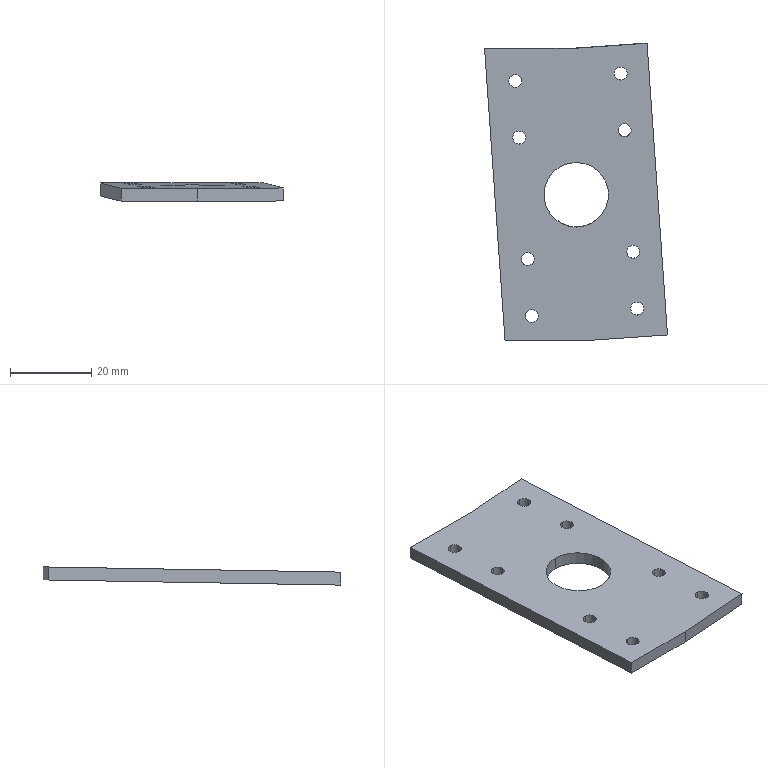Part | SolidWorks | features BaseBody 1 | 1 solid | 26 faces | box 45.033 x 73.349 x 4.479 mm | volume 8385 mm3 | cylinder 18 | plane 8 | commonest cylinder face diameters 3.2 x16 15.9 x2
STEP:
#1=CARTESIAN_POINT('',(17.015,-2.731,-4.048));
#2=VERTEX_POINT('',#1);
#3=CARTESIAN_POINT('',(17.015,0.4687,-3.992));
#4=VERTEX_POINT('',#3);
#5=CARTESIAN_POINT('',(17.015,-1.131,-4.02));
#6=DIRECTION('',(0.,0.01745,-0.9998));
#7=DIRECTION('',(0.,-0.9998,-0.01745));
#8=AXIS2_PLACEMENT_3D('',#5,#6,#7);
#9=CIRCLE('',#8,1.6);
#10=EDGE_CURVE('',#2,#4,#9,.T.);
#11=ORIENTED_EDGE('',*,*,#10,.T.);
#12=CARTESIAN_POINT('',(17.015,0.4129,-0.7929));
#13=VERTEX_POINT('',#12);
#14=CARTESIAN_POINT('',(17.015,0.4687,-3.992));
#15=DIRECTION('',(0.,-0.01745,0.9998));
#16=VECTOR('',#15,1000.);
#17=LINE('',#14,#16);
#18=EDGE_CURVE('',#4,#13,#17,.T.);
#19=ORIENTED_EDGE('',*,*,#18,.T.);
#20=CARTESIAN_POINT('',(17.015,-2.787,-0.8488));
#21=VERTEX_POINT('',#20);
#22=CARTESIAN_POINT('',(17.015,-1.187,-0.8208));
#23=DIRECTION('',(0.,-0.01745,0.9998));
#24=DIRECTION('',(0.,-0.9998,-0.01745));
#25=AXIS2_PLACEMENT_3D('',#22,#23,#24);
#26=CIRCLE('',#25,1.6);
#27=EDGE_CURVE('',#13,#21,#26,.T.);
#28=ORIENTED_EDGE('',*,*,#27,.T.);
#29=CARTESIAN_POINT('',(17.015,-2.731,-4.048));
#30=DIRECTION('',(0.,-0.01745,0.9998));
#31=VECTOR('',#30,1000.);
#32=LINE('',#29,#31);
#33=EDGE_CURVE('',#2,#21,#32,.T.);
#34=ORIENTED_EDGE('',*,*,#33,.F.);
#35=EDGE_LOOP('',(#11,#19,#28,#34));
#36=FACE_OUTER_BOUND('',#35,.T.);
#37=CARTESIAN_POINT('',(17.015,-1.131,-4.02));
#38=DIRECTION('',(0.,-0.01745,0.9998));
#39=DIRECTION('',(0.,-0.9998,-0.01745));
#40=AXIS2_PLACEMENT_3D('',#37,#38,#39);
#41=CYLINDRICAL_SURFACE('',#40,1.6);
#42=ADVANCED_FACE('',(#36),#41,.F.);
#43=CARTESIAN_POINT('',(-7.944,-15.31,-4.268));
#44=VERTEX_POINT('',#43);
#45=CARTESIAN_POINT('',(-7.944,-18.51,-4.324));
#46=VERTEX_POINT('',#45);
#47=CARTESIAN_POINT('',(-7.944,-16.91,-4.296));
#48=DIRECTION('',(0.,-0.01745,0.9998));
#49=DIRECTION('',(0.,-0.9998,-0.01745));
#50=AXIS2_PLACEMENT_3D('',#47,#48,#49);
#51=CIRCLE('',#50,1.6);
#52=EDGE_CURVE('',#44,#46,#51,.T.);
#53=ORIENTED_EDGE('',*,*,#52,.F.);
#54=CARTESIAN_POINT('',(-7.944,-15.366,-1.068));
#55=VERTEX_POINT('',#54);
#56=CARTESIAN_POINT('',(-7.944,-15.31,-4.268));
#57=DIRECTION('',(0.,-0.01745,0.9998));
#58=VECTOR('',#57,1000.);
#59=LINE('',#56,#58);
#60=EDGE_CURVE('',#44,#55,#59,.T.);
#61=ORIENTED_EDGE('',*,*,#60,.T.);
#62=CARTESIAN_POINT('',(-7.944,-18.565,-1.124));
#63=VERTEX_POINT('',#62);
#64=CARTESIAN_POINT('',(-7.944,-16.966,-1.096));
#65=DIRECTION('',(0.,-0.01745,0.9998));
#66=DIRECTION('',(0.,-0.9998,-0.01745));
#67=AXIS2_PLACEMENT_3D('',#64,#65,#66);
#68=CIRCLE('',#67,1.6);
#69=EDGE_CURVE('',#55,#63,#68,.T.);
#70=ORIENTED_EDGE('',*,*,#69,.T.);
#71=CARTESIAN_POINT('',(-7.944,-18.51,-4.324));
#72=DIRECTION('',(0.,-0.01745,0.9998));
#73=VECTOR('',#72,1000.);
#74=LINE('',#71,#73);
#75=EDGE_CURVE('',#46,#63,#74,.T.);
#76=ORIENTED_EDGE('',*,*,#75,.F.);
#77=EDGE_LOOP('',(#53,#61,#70,#76));
#78=FACE_OUTER_BOUND('',#77,.T.);
#79=CARTESIAN_POINT('',(-7.944,-16.91,-4.296));
#80=DIRECTION('',(0.,-0.01745,0.9998));
#81=DIRECTION('',(0.,-0.9998,-0.01745));
#82=AXIS2_PLACEMENT_3D('',#79,#80,#81);
#83=CYLINDRICAL_SURFACE('',#82,1.6);
#84=ADVANCED_FACE('',(#78),#83,.F.);
#85=CARTESIAN_POINT('',(3.,20.869,-3.636));
#86=VERTEX_POINT('',#85);
#87=CARTESIAN_POINT('',(3.,4.971,-3.914));
#88=VERTEX_POINT('',#87);
#89=CARTESIAN_POINT('',(3.,12.92,-3.775));
#90=DIRECTION('',(0.,-0.01745,0.9998));
#91=DIRECTION('',(0.,-0.9998,-0.01745));
#92=AXIS2_PLACEMENT_3D('',#89,#90,#91);
#93=CIRCLE('',#92,7.95);
#94=EDGE_CURVE('',#86,#88,#93,.T.);
#95=ORIENTED_EDGE('',*,*,#94,.F.);
#96=CARTESIAN_POINT('',(3.,20.813,-0.4368));
#97=VERTEX_POINT('',#96);
#98=CARTESIAN_POINT('',(3.,20.869,-3.636));
#99=DIRECTION('',(0.,-0.01745,0.9998));
#100=VECTOR('',#99,1000.);
#101=LINE('',#98,#100);
#102=EDGE_CURVE('',#86,#97,#101,.T.);
#103=ORIENTED_EDGE('',*,*,#102,.T.);
#104=CARTESIAN_POINT('',(3.,4.916,-0.7143));
#105=VERTEX_POINT('',#104);
#106=CARTESIAN_POINT('',(3.,12.864,-0.5756));
#107=DIRECTION('',(0.,-0.01745,0.9998));
#108=DIRECTION('',(0.,-0.9998,-0.01745));
#109=AXIS2_PLACEMENT_3D('',#106,#107,#108);
#110=CIRCLE('',#109,7.95);
#111=EDGE_CURVE('',#97,#105,#110,.T.);
#112=ORIENTED_EDGE('',*,*,#111,.T.);
#113=CARTESIAN_POINT('',(3.,4.971,-3.914));
#114=DIRECTION('',(0.,-0.01745,0.9998));
#115=VECTOR('',#114,1000.);
#116=LINE('',#113,#115);
#117=EDGE_CURVE('',#88,#105,#116,.T.);
#118=ORIENTED_EDGE('',*,*,#117,.F.);
#119=EDGE_LOOP('',(#95,#103,#112,#118));
#120=FACE_OUTER_BOUND('',#119,.T.);
#121=CARTESIAN_POINT('',(3.,12.92,-3.775));
#122=DIRECTION('',(0.,-0.01745,0.9998));
#123=DIRECTION('',(0.,-0.9998,-0.01745));
#124=AXIS2_PLACEMENT_3D('',#121,#122,#123);
#125=CYLINDRICAL_SURFACE('',#124,7.95);
#126=ADVANCED_FACE('',(#120),#125,.F.);
#127=CARTESIAN_POINT('',(-11.015,28.571,-3.502));
#128=VERTEX_POINT('',#127);
#129=CARTESIAN_POINT('',(-11.015,25.372,-3.558));
#130=VERTEX_POINT('',#129);
#131=CARTESIAN_POINT('',(-11.015,26.972,-3.53));
#132=DIRECTION('',(0.,-0.01745,0.9998));
#133=DIRECTION('',(0.,-0.9998,-0.01745));
#134=AXIS2_PLACEMENT_3D('',#131,#132,#133);
#135=CIRCLE('',#134,1.6);
#136=EDGE_CURVE('',#128,#130,#135,.T.);
#137=ORIENTED_EDGE('',*,*,#136,.F.);
#138=CARTESIAN_POINT('',(-11.015,28.515,-0.3024));
#139=VERTEX_POINT('',#138);
#140=CARTESIAN_POINT('',(-11.015,28.571,-3.502));
#141=DIRECTION('',(0.,-0.01745,0.9998));
#142=VECTOR('',#141,1000.);
#143=LINE('',#140,#142);
#144=EDGE_CURVE('',#128,#139,#143,.T.);
#145=ORIENTED_EDGE('',*,*,#144,.T.);
#146=CARTESIAN_POINT('',(-11.015,25.316,-0.3582));
#147=VERTEX_POINT('',#146);
#148=CARTESIAN_POINT('',(-11.015,26.916,-0.3303));
#149=DIRECTION('',(0.,-0.01745,0.9998));
#150=DIRECTION('',(0.,-0.9998,-0.01745));
#151=AXIS2_PLACEMENT_3D('',#148,#149,#150);
#152=CIRCLE('',#151,1.6);
#153=EDGE_CURVE('',#139,#147,#152,.T.);
#154=ORIENTED_EDGE('',*,*,#153,.T.);
#155=CARTESIAN_POINT('',(-11.015,25.372,-3.558));
#156=DIRECTION('',(0.,-0.01745,0.9998));
#157=VECTOR('',#156,1000.);
#158=LINE('',#155,#157);
#159=EDGE_CURVE('',#130,#147,#158,.T.);
#160=ORIENTED_EDGE('',*,*,#159,.F.);
#161=EDGE_LOOP('',(#137,#145,#154,#160));
#162=FACE_OUTER_BOUND('',#161,.T.);
#163=CARTESIAN_POINT('',(-11.015,26.972,-3.53));
#164=DIRECTION('',(0.,-0.01745,0.9998));
#165=DIRECTION('',(0.,-0.9998,-0.01745));
#166=AXIS2_PLACEMENT_3D('',#163,#164,#165);
#167=CYLINDRICAL_SURFACE('',#166,1.6);
#168=ADVANCED_FACE('',(#162),#167,.F.);
#169=CARTESIAN_POINT('',(13.944,44.35,-3.226));
#170=VERTEX_POINT('',#169);
#171=CARTESIAN_POINT('',(13.944,41.151,-3.282));
#172=VERTEX_POINT('',#171);
#173=CARTESIAN_POINT('',(13.944,42.75,-3.254));
#174=DIRECTION('',(0.,-0.01745,0.9998));
#175=DIRECTION('',(0.,-0.9998,-0.01745));
#176=AXIS2_PLACEMENT_3D('',#173,#174,#175);
#177=CIRCLE('',#176,1.6);
#178=EDGE_CURVE('',#170,#172,#177,.T.);
#179=ORIENTED_EDGE('',*,*,#178,.F.);
#180=CARTESIAN_POINT('',(13.944,44.294,-0.02696));
#181=VERTEX_POINT('',#180);
#182=CARTESIAN_POINT('',(13.944,44.35,-3.226));
#183=DIRECTION('',(0.,-0.01745,0.9998));
#184=VECTOR('',#183,1000.);
#185=LINE('',#182,#184);
#186=EDGE_CURVE('',#170,#181,#185,.T.);
#187=ORIENTED_EDGE('',*,*,#186,.T.);
#188=CARTESIAN_POINT('',(13.944,41.095,-0.08281));
#189=VERTEX_POINT('',#188);
#190=CARTESIAN_POINT('',(13.944,42.695,-0.05489));
#191=DIRECTION('',(0.,-0.01745,0.9998));
#192=DIRECTION('',(0.,-0.9998,-0.01745));
#193=AXIS2_PLACEMENT_3D('',#190,#191,#192);
#194=CIRCLE('',#193,1.6);
#195=EDGE_CURVE('',#181,#189,#194,.T.);
#196=ORIENTED_EDGE('',*,*,#195,.T.);
#197=CARTESIAN_POINT('',(13.944,41.151,-3.282));
#198=DIRECTION('',(0.,-0.01745,0.9998));
#199=VECTOR('',#198,1000.);
#200=LINE('',#197,#199);
#201=EDGE_CURVE('',#172,#189,#200,.T.);
#202=ORIENTED_EDGE('',*,*,#201,.F.);
#203=EDGE_LOOP('',(#179,#187,#196,#202));
#204=FACE_OUTER_BOUND('',#203,.T.);
#205=CARTESIAN_POINT('',(13.944,42.75,-3.254));
#206=DIRECTION('',(0.,-0.01745,0.9998));
#207=DIRECTION('',(0.,-0.9998,-0.01745));
#208=AXIS2_PLACEMENT_3D('',#205,#206,#207);
#209=CYLINDRICAL_SURFACE('',#208,1.6);
#210=ADVANCED_FACE('',(#204),#209,.F.);
#211=CARTESIAN_POINT('',(-11.993,42.535,-3.258));
#212=VERTEX_POINT('',#211);
#213=CARTESIAN_POINT('',(-11.993,39.336,-3.314));
#214=VERTEX_POINT('',#213);
#215=CARTESIAN_POINT('',(-11.993,40.935,-3.286));
#216=DIRECTION('',(0.,-0.01745,0.9998));
#217=DIRECTION('',(0.,-0.9998,-0.01745));
#218=AXIS2_PLACEMENT_3D('',#215,#216,#217);
#219=CIRCLE('',#218,1.6);
#220=EDGE_CURVE('',#212,#214,#219,.T.);
#221=ORIENTED_EDGE('',*,*,#220,.F.);
#222=CARTESIAN_POINT('',(-11.993,42.479,-0.05864));
#223=VERTEX_POINT('',#222);
#224=CARTESIAN_POINT('',(-11.993,42.535,-3.258));
#225=DIRECTION('',(0.,-0.01745,0.9998));
#226=VECTOR('',#225,1000.);
#227=LINE('',#224,#226);
#228=EDGE_CURVE('',#212,#223,#227,.T.);
#229=ORIENTED_EDGE('',*,*,#228,.T.);
#230=CARTESIAN_POINT('',(-11.993,39.28,-0.1145));
#231=VERTEX_POINT('',#230);
#232=CARTESIAN_POINT('',(-11.993,40.879,-0.08657));
#233=DIRECTION('',(0.,-0.01745,0.9998));
#234=DIRECTION('',(0.,-0.9998,-0.01745));
#235=AXIS2_PLACEMENT_3D('',#232,#233,#234);
#236=CIRCLE('',#235,1.6);
#237=EDGE_CURVE('',#223,#231,#236,.T.);
#238=ORIENTED_EDGE('',*,*,#237,.T.);
#239=CARTESIAN_POINT('',(-11.993,39.336,-3.314));
#240=DIRECTION('',(0.,-0.01745,0.9998));
#241=VECTOR('',#240,1000.);
#242=LINE('',#239,#241);
#243=EDGE_CURVE('',#214,#231,#242,.T.);
#244=ORIENTED_EDGE('',*,*,#243,.F.);
#245=EDGE_LOOP('',(#221,#229,#238,#244));
#246=FACE_OUTER_BOUND('',#245,.T.);
#247=CARTESIAN_POINT('',(-11.993,40.935,-3.286));
#248=DIRECTION('',(0.,-0.01745,0.9998));
#249=DIRECTION('',(0.,-0.9998,-0.01745));
#250=AXIS2_PLACEMENT_3D('',#247,#248,#249);
#251=CYLINDRICAL_SURFACE('',#250,1.6);
#252=ADVANCED_FACE('',(#246),#251,.F.);
#253=CARTESIAN_POINT('',(14.921,30.386,-3.47));
#254=VERTEX_POINT('',#253);
#255=CARTESIAN_POINT('',(14.921,27.187,-3.526));
#256=VERTEX_POINT('',#255);
#257=CARTESIAN_POINT('',(14.921,28.787,-3.498));
#258=DIRECTION('',(0.,-0.01745,0.9998));
#259=DIRECTION('',(0.,-0.9998,-0.01745));
#260=AXIS2_PLACEMENT_3D('',#257,#258,#259);
#261=CIRCLE('',#260,1.6);
#262=EDGE_CURVE('',#254,#256,#261,.T.);
#263=ORIENTED_EDGE('',*,*,#262,.F.);
#264=CARTESIAN_POINT('',(14.921,30.331,-0.2707));
#265=VERTEX_POINT('',#264);
#266=CARTESIAN_POINT('',(14.921,30.386,-3.47));
#267=DIRECTION('',(0.,-0.01745,0.9998));
#268=VECTOR('',#267,1000.);
#269=LINE('',#266,#268);
#270=EDGE_CURVE('',#254,#265,#269,.T.);
#271=ORIENTED_EDGE('',*,*,#270,.T.);
#272=CARTESIAN_POINT('',(14.921,27.131,-0.3265));
#273=VERTEX_POINT('',#272);
#274=CARTESIAN_POINT('',(14.921,28.731,-0.2986));
#275=DIRECTION('',(0.,-0.01745,0.9998));
#276=DIRECTION('',(0.,-0.9998,-0.01745));
#277=AXIS2_PLACEMENT_3D('',#274,#275,#276);
#278=CIRCLE('',#277,1.6);
#279=EDGE_CURVE('',#265,#273,#278,.T.);
#280=ORIENTED_EDGE('',*,*,#279,.T.);
#281=CARTESIAN_POINT('',(14.921,27.187,-3.526));
#282=DIRECTION('',(0.,-0.01745,0.9998));
#283=VECTOR('',#282,1000.);
#284=LINE('',#281,#283);
#285=EDGE_CURVE('',#256,#273,#284,.T.);
#286=ORIENTED_EDGE('',*,*,#285,.F.);
#287=EDGE_LOOP('',(#263,#271,#280,#286));
#288=FACE_OUTER_BOUND('',#287,.T.);
#289=CARTESIAN_POINT('',(14.921,28.787,-3.498));
#290=DIRECTION('',(0.,-0.01745,0.9998));
#291=DIRECTION('',(0.,-0.9998,-0.01745));
#292=AXIS2_PLACEMENT_3D('',#289,#290,#291);
#293=CYLINDRICAL_SURFACE('',#292,1.6);
#294=ADVANCED_FACE('',(#288),#293,.F.);
#295=CARTESIAN_POINT('',(-8.921,-1.346,-4.024));
#296=VERTEX_POINT('',#295);
#297=CARTESIAN_POINT('',(-8.921,-4.546,-4.08));
#298=VERTEX_POINT('',#297);
#299=CARTESIAN_POINT('',(-8.921,-2.946,-4.052));
#300=DIRECTION('',(0.,-0.01745,0.9998));
#301=DIRECTION('',(0.,-0.9998,-0.01745));
#302=AXIS2_PLACEMENT_3D('',#299,#300,#301);
#303=CIRCLE('',#302,1.6);
#304=EDGE_CURVE('',#296,#298,#303,.T.);
#305=ORIENTED_EDGE('',*,*,#304,.F.);
#306=CARTESIAN_POINT('',(-8.921,-1.402,-0.8246));
#307=VERTEX_POINT('',#306);
#308=CARTESIAN_POINT('',(-8.921,-1.346,-4.024));
#309=DIRECTION('',(0.,-0.01745,0.9998));
#310=VECTOR('',#309,1000.);
#311=LINE('',#308,#310);
#312=EDGE_CURVE('',#296,#307,#311,.T.);
#313=ORIENTED_EDGE('',*,*,#312,.T.);
#314=CARTESIAN_POINT('',(-8.921,-4.602,-0.8804));
#315=VERTEX_POINT('',#314);
#316=CARTESIAN_POINT('',(-8.921,-3.002,-0.8525));
#317=DIRECTION('',(0.,-0.01745,0.9998));
#318=DIRECTION('',(0.,-0.9998,-0.01745));
#319=AXIS2_PLACEMENT_3D('',#316,#317,#318);
#320=CIRCLE('',#319,1.6);
#321=EDGE_CURVE('',#307,#315,#320,.T.);
#322=ORIENTED_EDGE('',*,*,#321,.T.);
#323=CARTESIAN_POINT('',(-8.921,-4.546,-4.08));
#324=DIRECTION('',(0.,-0.01745,0.9998));
#325=VECTOR('',#324,1000.);
#326=LINE('',#323,#325);
#327=EDGE_CURVE('',#298,#315,#326,.T.);
#328=ORIENTED_EDGE('',*,*,#327,.F.);
#329=EDGE_LOOP('',(#305,#313,#322,#328));
#330=FACE_OUTER_BOUND('',#329,.T.);
#331=CARTESIAN_POINT('',(-8.921,-2.946,-4.052));
#332=DIRECTION('',(0.,-0.01745,0.9998));
#333=DIRECTION('',(0.,-0.9998,-0.01745));
#334=AXIS2_PLACEMENT_3D('',#331,#332,#333);
#335=CYLINDRICAL_SURFACE('',#334,1.6);
#336=ADVANCED_FACE('',(#330),#335,.F.);
#337=CARTESIAN_POINT('',(17.993,-13.495,-4.236));
#338=VERTEX_POINT('',#337);
#339=CARTESIAN_POINT('',(17.993,-16.694,-4.292));
#340=VERTEX_POINT('',#339);
#341=CARTESIAN_POINT('',(17.993,-15.095,-4.264));
#342=DIRECTION('',(0.,-0.01745,0.9998));
#343=DIRECTION('',(0.,-0.9998,-0.01745));
#344=AXIS2_PLACEMENT_3D('',#341,#342,#343);
#345=CIRCLE('',#344,1.6);
#346=EDGE_CURVE('',#338,#340,#345,.T.);
#347=ORIENTED_EDGE('',*,*,#346,.F.);
#348=CARTESIAN_POINT('',(17.993,-13.551,-1.037));
#349=VERTEX_POINT('',#348);
#350=CARTESIAN_POINT('',(17.993,-13.495,-4.236));
#351=DIRECTION('',(0.,-0.01745,0.9998));
#352=VECTOR('',#351,1000.);
#353=LINE('',#350,#352);
#354=EDGE_CURVE('',#338,#349,#353,.T.);
#355=ORIENTED_EDGE('',*,*,#354,.T.);
#356=CARTESIAN_POINT('',(17.993,-16.75,-1.093));
#357=VERTEX_POINT('',#356);
#358=CARTESIAN_POINT('',(17.993,-15.151,-1.065));
#359=DIRECTION('',(0.,-0.01745,0.9998));
#360=DIRECTION('',(0.,-0.9998,-0.01745));
#361=AXIS2_PLACEMENT_3D('',#358,#359,#360);
#362=CIRCLE('',#361,1.6);
#363=EDGE_CURVE('',#349,#357,#362,.T.);
#364=ORIENTED_EDGE('',*,*,#363,.T.);
#365=CARTESIAN_POINT('',(17.993,-16.694,-4.292));
#366=DIRECTION('',(0.,-0.01745,0.9998));
#367=VECTOR('',#366,1000.);
#368=LINE('',#365,#367);
#369=EDGE_CURVE('',#340,#357,#368,.T.);
#370=ORIENTED_EDGE('',*,*,#369,.F.);
#371=EDGE_LOOP('',(#347,#355,#364,#370));
#372=FACE_OUTER_BOUND('',#371,.T.);
#373=CARTESIAN_POINT('',(17.993,-15.095,-4.264));
#374=DIRECTION('',(0.,-0.01745,0.9998));
#375=DIRECTION('',(0.,-0.9998,-0.01745));
#376=AXIS2_PLACEMENT_3D('',#373,#374,#375);
#377=CYLINDRICAL_SURFACE('',#376,1.6);
#378=ADVANCED_FACE('',(#372),#377,.F.);
#379=ORIENTED_EDGE('',*,*,#18,.F.);
#380=CARTESIAN_POINT('',(17.015,-1.131,-4.02));
#381=DIRECTION('',(0.,0.01745,-0.9998));
#382=DIRECTION('',(0.,-0.9998,-0.01745));
#383=AXIS2_PLACEMENT_3D('',#380,#381,#382);
#384=CIRCLE('',#383,1.6);
#385=EDGE_CURVE('',#4,#2,#384,.T.);
#386=ORIENTED_EDGE('',*,*,#385,.T.);
#387=ORIENTED_EDGE('',*,*,#33,.T.);
#388=CARTESIAN_POINT('',(17.015,-1.187,-0.8208));
#389=DIRECTION('',(0.,-0.01745,0.9998));
#390=DIRECTION('',(0.,-0.9998,-0.01745));
#391=AXIS2_PLACEMENT_3D('',#388,#389,#390);
#392=CIRCLE('',#391,1.6);
#393=EDGE_CURVE('',#21,#13,#392,.T.);
#394=ORIENTED_EDGE('',*,*,#393,.T.);
#395=EDGE_LOOP('',(#379,#386,#387,#394));
#396=FACE_OUTER_BOUND('',#395,.T.);
#397=CARTESIAN_POINT('',(17.015,-1.131,-4.02));
#398=DIRECTION('',(0.,-0.01745,0.9998));
#399=DIRECTION('',(0.,-0.9998,-0.01745));
#400=AXIS2_PLACEMENT_3D('',#397,#398,#399);
#401=CYLINDRICAL_SURFACE('',#400,1.6);
#402=ADVANCED_FACE('',(#396),#401,.F.);
#403=ORIENTED_EDGE('',*,*,#393,.F.);
#404=ORIENTED_EDGE('',*,*,#27,.F.);
#405=EDGE_LOOP('',(#403,#404));
#406=FACE_BOUND('',#405,.T.);
#407=CARTESIAN_POINT('',(-7.944,-16.966,-1.096));
#408=DIRECTION('',(0.,-0.01745,0.9998));
#409=DIRECTION('',(0.,-0.9998,-0.01745));
#410=AXIS2_PLACEMENT_3D('',#407,#408,#409);
#411=CIRCLE('',#410,1.6);
#412=EDGE_CURVE('',#63,#55,#411,.T.);
#413=ORIENTED_EDGE('',*,*,#412,.F.);
#414=ORIENTED_EDGE('',*,*,#69,.F.);
#415=EDGE_LOOP('',(#413,#414));
#416=FACE_BOUND('',#415,.T.);
#417=CARTESIAN_POINT('',(3.,12.864,-0.5756));
#418=DIRECTION('',(0.,-0.01745,0.9998));
#419=DIRECTION('',(0.,-0.9998,-0.01745));
#420=AXIS2_PLACEMENT_3D('',#417,#418,#419);
#421=CIRCLE('',#420,7.95);
#422=EDGE_CURVE('',#105,#97,#421,.T.);
#423=ORIENTED_EDGE('',*,*,#422,.F.);
#424=ORIENTED_EDGE('',*,*,#111,.F.);
#425=EDGE_LOOP('',(#423,#424));
#426=FACE_BOUND('',#425,.T.);
#427=CARTESIAN_POINT('',(-11.015,26.916,-0.3303));
#428=DIRECTION('',(0.,-0.01745,0.9998));
#429=DIRECTION('',(0.,-0.9998,-0.01745));
#430=AXIS2_PLACEMENT_3D('',#427,#428,#429);
#431=CIRCLE('',#430,1.6);
#432=EDGE_CURVE('',#147,#139,#431,.T.);
#433=ORIENTED_EDGE('',*,*,#432,.F.);
#434=ORIENTED_EDGE('',*,*,#153,.F.);
#435=EDGE_LOOP('',(#433,#434));
#436=FACE_BOUND('',#435,.T.);
#437=CARTESIAN_POINT('',(13.944,42.695,-0.05489));
#438=DIRECTION('',(0.,-0.01745,0.9998));
#439=DIRECTION('',(0.,-0.9998,-0.01745));
#440=AXIS2_PLACEMENT_3D('',#437,#438,#439);
#441=CIRCLE('',#440,1.6);
#442=EDGE_CURVE('',#189,#181,#441,.T.);
#443=ORIENTED_EDGE('',*,*,#442,.F.);
#444=ORIENTED_EDGE('',*,*,#195,.F.);
#445=EDGE_LOOP('',(#443,#444));
#446=FACE_BOUND('',#445,.T.);
#447=CARTESIAN_POINT('',(-11.993,40.879,-0.08657));
#448=DIRECTION('',(0.,-0.01745,0.9998));
#449=DIRECTION('',(0.,-0.9998,-0.01745));
#450=AXIS2_PLACEMENT_3D('',#447,#448,#449);
#451=CIRCLE('',#450,1.6);
#452=EDGE_CURVE('',#231,#223,#451,.T.);
#453=ORIENTED_EDGE('',*,*,#452,.F.);
#454=ORIENTED_EDGE('',*,*,#237,.F.);
#455=EDGE_LOOP('',(#453,#454));
#456=FACE_BOUND('',#455,.T.);
#457=CARTESIAN_POINT('',(14.921,28.731,-0.2986));
#458=DIRECTION('',(0.,-0.01745,0.9998));
#459=DIRECTION('',(0.,-0.9998,-0.01745));
#460=AXIS2_PLACEMENT_3D('',#457,#458,#459);
#461=CIRCLE('',#460,1.6);
#462=EDGE_CURVE('',#273,#265,#461,.T.);
#463=ORIENTED_EDGE('',*,*,#462,.F.);
#464=ORIENTED_EDGE('',*,*,#279,.F.);
#465=EDGE_LOOP('',(#463,#464));
#466=FACE_BOUND('',#465,.T.);
#467=CARTESIAN_POINT('',(-8.921,-3.002,-0.8525));
#468=DIRECTION('',(0.,-0.01745,0.9998));
#469=DIRECTION('',(0.,-0.9998,-0.01745));
#470=AXIS2_PLACEMENT_3D('',#467,#468,#469);
#471=CIRCLE('',#470,1.6);
#472=EDGE_CURVE('',#315,#307,#471,.T.);
#473=ORIENTED_EDGE('',*,*,#472,.F.);
#474=ORIENTED_EDGE('',*,*,#321,.F.);
#475=EDGE_LOOP('',(#473,#474));
#476=FACE_BOUND('',#475,.T.);
#477=CARTESIAN_POINT('',(17.993,-15.151,-1.065));
#478=DIRECTION('',(0.,-0.01745,0.9998));
#479=DIRECTION('',(0.,-0.9998,-0.01745));
#480=AXIS2_PLACEMENT_3D('',#477,#478,#479);
#481=CIRCLE('',#480,1.6);
#482=EDGE_CURVE('',#357,#349,#481,.T.);
#483=ORIENTED_EDGE('',*,*,#482,.F.);
#484=ORIENTED_EDGE('',*,*,#363,.F.);
#485=EDGE_LOOP('',(#483,#484));
#486=FACE_BOUND('',#485,.T.);
#487=CARTESIAN_POINT('',(20.438,50.165,0.07551));
#488=VERTEX_POINT('',#487);
#489=CARTESIAN_POINT('',(25.465,-21.644,-1.178));
#490=VERTEX_POINT('',#489);
#491=CARTESIAN_POINT('',(20.438,50.165,0.07551));
#492=DIRECTION('',(0.06982,-0.9974,-0.01741));
#493=VECTOR('',#492,1000.);
#494=LINE('',#491,#493);
#495=EDGE_CURVE('',#488,#490,#494,.T.);
#496=ORIENTED_EDGE('',*,*,#495,.F.);
#497=CARTESIAN_POINT('',(1.742,48.857,0.05267));
#498=VERTEX_POINT('',#497);
#499=CARTESIAN_POINT('',(1.742,48.857,0.05267));
#500=DIRECTION('',(0.9976,0.06981,0.001219));
#501=VECTOR('',#500,1000.);
#502=LINE('',#499,#501);
#503=EDGE_CURVE('',#498,#488,#502,.T.);
#504=ORIENTED_EDGE('',*,*,#503,.F.);
#505=CARTESIAN_POINT('',(-19.568,48.857,0.05267));
#506=VERTEX_POINT('',#505);
#507=CARTESIAN_POINT('',(2.948,48.857,0.05267));
#508=DIRECTION('',(1.,0.,0.));
#509=VECTOR('',#508,1000.);
#510=LINE('',#507,#509);
#511=EDGE_CURVE('',#506,#498,#510,.T.);
#512=ORIENTED_EDGE('',*,*,#511,.F.);
#513=CARTESIAN_POINT('',(-14.529,-23.128,-1.204));
#514=VERTEX_POINT('',#513);
#515=CARTESIAN_POINT('',(-14.529,-23.128,-1.204));
#516=DIRECTION('',(-0.06982,0.9974,0.01741));
#517=VECTOR('',#516,1000.);
#518=LINE('',#515,#517);
#519=EDGE_CURVE('',#514,#506,#518,.T.);
#520=ORIENTED_EDGE('',*,*,#519,.F.);
#521=CARTESIAN_POINT('',(4.258,-23.128,-1.204));
#522=VERTEX_POINT('',#521);
#523=CARTESIAN_POINT('',(2.948,-23.128,-1.204));
#524=DIRECTION('',(-1.,0.,0.));
#525=VECTOR('',#524,1000.);
#526=LINE('',#523,#525);
#527=EDGE_CURVE('',#522,#514,#526,.T.);
#528=ORIENTED_EDGE('',*,*,#527,.F.);
#529=CARTESIAN_POINT('',(25.465,-21.644,-1.178));
#530=DIRECTION('',(-0.9976,-0.06981,-0.001219));
#531=VECTOR('',#530,1000.);
#532=LINE('',#529,#531);
#533=EDGE_CURVE('',#490,#522,#532,.T.);
#534=ORIENTED_EDGE('',*,*,#533,.F.);
#535=EDGE_LOOP('',(#496,#504,#512,#520,#528,#534));
#536=FACE_OUTER_BOUND('',#535,.T.);
#537=CARTESIAN_POINT('',(-19.839,-23.128,-1.204));
#538=DIRECTION('',(0.,0.01745,-0.9998));
#539=DIRECTION('',(0.,0.9998,0.01745));
#540=AXIS2_PLACEMENT_3D('',#537,#538,#539);
#541=PLANE('',#540);
#542=ADVANCED_FACE('',(#406,#416,#426,#436,#446,#456,#466,#476,#486,#536),#541,.F.);
#543=ORIENTED_EDGE('',*,*,#10,.F.);
#544=ORIENTED_EDGE('',*,*,#385,.F.);
#545=EDGE_LOOP('',(#543,#544));
#546=FACE_BOUND('',#545,.T.);
#547=CARTESIAN_POINT('',(-7.944,-16.91,-4.296));
#548=DIRECTION('',(0.,-0.01745,0.9998));
#549=DIRECTION('',(0.,-0.9998,-0.01745));
#550=AXIS2_PLACEMENT_3D('',#547,#548,#549);
#551=CIRCLE('',#550,1.6);
#552=EDGE_CURVE('',#46,#44,#551,.T.);
#553=ORIENTED_EDGE('',*,*,#552,.T.);
#554=ORIENTED_EDGE('',*,*,#52,.T.);
#555=EDGE_LOOP('',(#553,#554));
#556=FACE_BOUND('',#555,.T.);
#557=CARTESIAN_POINT('',(3.,12.92,-3.775));
#558=DIRECTION('',(0.,-0.01745,0.9998));
#559=DIRECTION('',(0.,-0.9998,-0.01745));
#560=AXIS2_PLACEMENT_3D('',#557,#558,#559);
#561=CIRCLE('',#560,7.95);
#562=EDGE_CURVE('',#88,#86,#561,.T.);
#563=ORIENTED_EDGE('',*,*,#562,.T.);
#564=ORIENTED_EDGE('',*,*,#94,.T.);
#565=EDGE_LOOP('',(#563,#564));
#566=FACE_BOUND('',#565,.T.);
#567=CARTESIAN_POINT('',(-11.015,26.972,-3.53));
#568=DIRECTION('',(0.,-0.01745,0.9998));
#569=DIRECTION('',(0.,-0.9998,-0.01745));
#570=AXIS2_PLACEMENT_3D('',#567,#568,#569);
#571=CIRCLE('',#570,1.6);
#572=EDGE_CURVE('',#130,#128,#571,.T.);
#573=ORIENTED_EDGE('',*,*,#572,.T.);
#574=ORIENTED_EDGE('',*,*,#136,.T.);
#575=EDGE_LOOP('',(#573,#574));
#576=FACE_BOUND('',#575,.T.);
#577=CARTESIAN_POINT('',(13.944,42.75,-3.254));
#578=DIRECTION('',(0.,-0.01745,0.9998));
#579=DIRECTION('',(0.,-0.9998,-0.01745));
#580=AXIS2_PLACEMENT_3D('',#577,#578,#579);
#581=CIRCLE('',#580,1.6);
#582=EDGE_CURVE('',#172,#170,#581,.T.);
#583=ORIENTED_EDGE('',*,*,#582,.T.);
#584=ORIENTED_EDGE('',*,*,#178,.T.);
#585=EDGE_LOOP('',(#583,#584));
#586=FACE_BOUND('',#585,.T.);
#587=CARTESIAN_POINT('',(-11.993,40.935,-3.286));
#588=DIRECTION('',(0.,-0.01745,0.9998));
#589=DIRECTION('',(0.,-0.9998,-0.01745));
#590=AXIS2_PLACEMENT_3D('',#587,#588,#589);
#591=CIRCLE('',#590,1.6);
#592=EDGE_CURVE('',#214,#212,#591,.T.);
#593=ORIENTED_EDGE('',*,*,#592,.T.);
#594=ORIENTED_EDGE('',*,*,#220,.T.);
#595=EDGE_LOOP('',(#593,#594));
#596=FACE_BOUND('',#595,.T.);
#597=CARTESIAN_POINT('',(14.921,28.787,-3.498));
#598=DIRECTION('',(0.,-0.01745,0.9998));
#599=DIRECTION('',(0.,-0.9998,-0.01745));
#600=AXIS2_PLACEMENT_3D('',#597,#598,#599);
#601=CIRCLE('',#600,1.6);
#602=EDGE_CURVE('',#256,#254,#601,.T.);
#603=ORIENTED_EDGE('',*,*,#602,.T.);
#604=ORIENTED_EDGE('',*,*,#262,.T.);
#605=EDGE_LOOP('',(#603,#604));
#606=FACE_BOUND('',#605,.T.);
#607=CARTESIAN_POINT('',(-8.921,-2.946,-4.052));
#608=DIRECTION('',(0.,-0.01745,0.9998));
#609=DIRECTION('',(0.,-0.9998,-0.01745));
#610=AXIS2_PLACEMENT_3D('',#607,#608,#609);
#611=CIRCLE('',#610,1.6);
#612=EDGE_CURVE('',#298,#296,#611,.T.);
#613=ORIENTED_EDGE('',*,*,#612,.T.);
#614=ORIENTED_EDGE('',*,*,#304,.T.);
#615=EDGE_LOOP('',(#613,#614));
#616=FACE_BOUND('',#615,.T.);
#617=CARTESIAN_POINT('',(17.993,-15.095,-4.264));
#618=DIRECTION('',(0.,-0.01745,0.9998));
#619=DIRECTION('',(0.,-0.9998,-0.01745));
#620=AXIS2_PLACEMENT_3D('',#617,#618,#619);
#621=CIRCLE('',#620,1.6);
#622=EDGE_CURVE('',#340,#338,#621,.T.);
#623=ORIENTED_EDGE('',*,*,#622,.T.);
#624=ORIENTED_EDGE('',*,*,#346,.T.);
#625=EDGE_LOOP('',(#623,#624));
#626=FACE_BOUND('',#625,.T.);
#627=CARTESIAN_POINT('',(1.742,48.913,-3.147));
#628=VERTEX_POINT('',#627);
#629=CARTESIAN_POINT('',(20.438,50.221,-3.124));
#630=VERTEX_POINT('',#629);
#631=CARTESIAN_POINT('',(1.742,48.913,-3.147));
#632=DIRECTION('',(0.9976,0.06981,0.001219));
#633=VECTOR('',#632,1000.);
#634=LINE('',#631,#633);
#635=EDGE_CURVE('',#628,#630,#634,.T.);
#636=ORIENTED_EDGE('',*,*,#635,.T.);
#637=CARTESIAN_POINT('',(25.465,-21.588,-4.377));
#638=VERTEX_POINT('',#637);
#639=CARTESIAN_POINT('',(20.438,50.221,-3.124));
#640=DIRECTION('',(0.06982,-0.9974,-0.01741));
#641=VECTOR('',#640,1000.);
#642=LINE('',#639,#641);
#643=EDGE_CURVE('',#630,#638,#642,.T.);
#644=ORIENTED_EDGE('',*,*,#643,.T.);
#645=CARTESIAN_POINT('',(4.258,-23.072,-4.403));
#646=VERTEX_POINT('',#645);
#647=CARTESIAN_POINT('',(25.465,-21.588,-4.377));
#648=DIRECTION('',(-0.9976,-0.06981,-0.001219));
#649=VECTOR('',#648,1000.);
#650=LINE('',#647,#649);
#651=EDGE_CURVE('',#638,#646,#650,.T.);
#652=ORIENTED_EDGE('',*,*,#651,.T.);
#653=CARTESIAN_POINT('',(-14.529,-23.072,-4.403));
#654=VERTEX_POINT('',#653);
#655=CARTESIAN_POINT('',(2.948,-23.072,-4.403));
#656=DIRECTION('',(-1.,0.,0.));
#657=VECTOR('',#656,1000.);
#658=LINE('',#655,#657);
#659=EDGE_CURVE('',#646,#654,#658,.T.);
#660=ORIENTED_EDGE('',*,*,#659,.T.);
#661=CARTESIAN_POINT('',(-19.568,48.913,-3.147));
#662=VERTEX_POINT('',#661);
#663=CARTESIAN_POINT('',(-14.529,-23.072,-4.403));
#664=DIRECTION('',(-0.06982,0.9974,0.01741));
#665=VECTOR('',#664,1000.);
#666=LINE('',#663,#665);
#667=EDGE_CURVE('',#654,#662,#666,.T.);
#668=ORIENTED_EDGE('',*,*,#667,.T.);
#669=CARTESIAN_POINT('',(2.948,48.913,-3.147));
#670=DIRECTION('',(1.,0.,0.));
#671=VECTOR('',#670,1000.);
#672=LINE('',#669,#671);
#673=EDGE_CURVE('',#662,#628,#672,.T.);
#674=ORIENTED_EDGE('',*,*,#673,.T.);
#675=EDGE_LOOP('',(#636,#644,#652,#660,#668,#674));
#676=FACE_OUTER_BOUND('',#675,.T.);
#677=CARTESIAN_POINT('',(-19.839,-23.072,-4.403));
#678=DIRECTION('',(0.,0.01745,-0.9998));
#679=DIRECTION('',(0.,0.9998,0.01745));
#680=AXIS2_PLACEMENT_3D('',#677,#678,#679);
#681=PLANE('',#680);
#682=ADVANCED_FACE('',(#546,#556,#566,#576,#586,#596,#606,#616,#626,#676),#681,.T.);
#683=ORIENTED_EDGE('',*,*,#60,.F.);
#684=ORIENTED_EDGE('',*,*,#552,.F.);
#685=ORIENTED_EDGE('',*,*,#75,.T.);
#686=ORIENTED_EDGE('',*,*,#412,.T.);
#687=EDGE_LOOP('',(#683,#684,#685,#686));
#688=FACE_OUTER_BOUND('',#687,.T.);
#689=CARTESIAN_POINT('',(-7.944,-16.91,-4.296));
#690=DIRECTION('',(0.,-0.01745,0.9998));
#691=DIRECTION('',(0.,-0.9998,-0.01745));
#692=AXIS2_PLACEMENT_3D('',#689,#690,#691);
#693=CYLINDRICAL_SURFACE('',#692,1.6);
#694=ADVANCED_FACE('',(#688),#693,.F.);
#695=ORIENTED_EDGE('',*,*,#102,.F.);
#696=ORIENTED_EDGE('',*,*,#562,.F.);
#697=ORIENTED_EDGE('',*,*,#117,.T.);
#698=ORIENTED_EDGE('',*,*,#422,.T.);
#699=EDGE_LOOP('',(#695,#696,#697,#698));
#700=FACE_OUTER_BOUND('',#699,.T.);
#701=CARTESIAN_POINT('',(3.,12.92,-3.775));
#702=DIRECTION('',(0.,-0.01745,0.9998));
#703=DIRECTION('',(0.,-0.9998,-0.01745));
#704=AXIS2_PLACEMENT_3D('',#701,#702,#703);
#705=CYLINDRICAL_SURFACE('',#704,7.95);
#706=ADVANCED_FACE('',(#700),#705,.F.);
#707=ORIENTED_EDGE('',*,*,#144,.F.);
#708=ORIENTED_EDGE('',*,*,#572,.F.);
#709=ORIENTED_EDGE('',*,*,#159,.T.);
#710=ORIENTED_EDGE('',*,*,#432,.T.);
#711=EDGE_LOOP('',(#707,#708,#709,#710));
#712=FACE_OUTER_BOUND('',#711,.T.);
#713=CARTESIAN_POINT('',(-11.015,26.972,-3.53));
#714=DIRECTION('',(0.,-0.01745,0.9998));
#715=DIRECTION('',(0.,-0.9998,-0.01745));
#716=AXIS2_PLACEMENT_3D('',#713,#714,#715);
#717=CYLINDRICAL_SURFACE('',#716,1.6);
#718=ADVANCED_FACE('',(#712),#717,.F.);
#719=ORIENTED_EDGE('',*,*,#186,.F.);
#720=ORIENTED_EDGE('',*,*,#582,.F.);
#721=ORIENTED_EDGE('',*,*,#201,.T.);
#722=ORIENTED_EDGE('',*,*,#442,.T.);
#723=EDGE_LOOP('',(#719,#720,#721,#722));
#724=FACE_OUTER_BOUND('',#723,.T.);
#725=CARTESIAN_POINT('',(13.944,42.75,-3.254));
#726=DIRECTION('',(0.,-0.01745,0.9998));
#727=DIRECTION('',(0.,-0.9998,-0.01745));
#728=AXIS2_PLACEMENT_3D('',#725,#726,#727);
#729=CYLINDRICAL_SURFACE('',#728,1.6);
#730=ADVANCED_FACE('',(#724),#729,.F.);
#731=ORIENTED_EDGE('',*,*,#228,.F.);
#732=ORIENTED_EDGE('',*,*,#592,.F.);
#733=ORIENTED_EDGE('',*,*,#243,.T.);
#734=ORIENTED_EDGE('',*,*,#452,.T.);
#735=EDGE_LOOP('',(#731,#732,#733,#734));
#736=FACE_OUTER_BOUND('',#735,.T.);
#737=CARTESIAN_POINT('',(-11.993,40.935,-3.286));
#738=DIRECTION('',(0.,-0.01745,0.9998));
#739=DIRECTION('',(0.,-0.9998,-0.01745));
#740=AXIS2_PLACEMENT_3D('',#737,#738,#739);
#741=CYLINDRICAL_SURFACE('',#740,1.6);
#742=ADVANCED_FACE('',(#736),#741,.F.);
#743=ORIENTED_EDGE('',*,*,#270,.F.);
#744=ORIENTED_EDGE('',*,*,#602,.F.);
#745=ORIENTED_EDGE('',*,*,#285,.T.);
#746=ORIENTED_EDGE('',*,*,#462,.T.);
#747=EDGE_LOOP('',(#743,#744,#745,#746));
#748=FACE_OUTER_BOUND('',#747,.T.);
#749=CARTESIAN_POINT('',(14.921,28.787,-3.498));
#750=DIRECTION('',(0.,-0.01745,0.9998));
#751=DIRECTION('',(0.,-0.9998,-0.01745));
#752=AXIS2_PLACEMENT_3D('',#749,#750,#751);
#753=CYLINDRICAL_SURFACE('',#752,1.6);
#754=ADVANCED_FACE('',(#748),#753,.F.);
#755=ORIENTED_EDGE('',*,*,#312,.F.);
#756=ORIENTED_EDGE('',*,*,#612,.F.);
#757=ORIENTED_EDGE('',*,*,#327,.T.);
#758=ORIENTED_EDGE('',*,*,#472,.T.);
#759=EDGE_LOOP('',(#755,#756,#757,#758));
#760=FACE_OUTER_BOUND('',#759,.T.);
#761=CARTESIAN_POINT('',(-8.921,-2.946,-4.052));
#762=DIRECTION('',(0.,-0.01745,0.9998));
#763=DIRECTION('',(0.,-0.9998,-0.01745));
#764=AXIS2_PLACEMENT_3D('',#761,#762,#763);
#765=CYLINDRICAL_SURFACE('',#764,1.6);
#766=ADVANCED_FACE('',(#760),#765,.F.);
#767=ORIENTED_EDGE('',*,*,#354,.F.);
#768=ORIENTED_EDGE('',*,*,#622,.F.);
#769=ORIENTED_EDGE('',*,*,#369,.T.);
#770=ORIENTED_EDGE('',*,*,#482,.T.);
#771=EDGE_LOOP('',(#767,#768,#769,#770));
#772=FACE_OUTER_BOUND('',#771,.T.);
#773=CARTESIAN_POINT('',(17.993,-15.095,-4.264));
#774=DIRECTION('',(0.,-0.01745,0.9998));
#775=DIRECTION('',(0.,-0.9998,-0.01745));
#776=AXIS2_PLACEMENT_3D('',#773,#774,#775);
#777=CYLINDRICAL_SURFACE('',#776,1.6);
#778=ADVANCED_FACE('',(#772),#777,.F.);
#779=CARTESIAN_POINT('',(4.258,-23.072,-4.403));
#780=DIRECTION('',(0.,-0.01745,0.9998));
#781=VECTOR('',#780,1000.);
#782=LINE('',#779,#781);
#783=EDGE_CURVE('',#646,#522,#782,.T.);
#784=ORIENTED_EDGE('',*,*,#783,.F.);
#785=ORIENTED_EDGE('',*,*,#651,.F.);
#786=CARTESIAN_POINT('',(25.465,-21.644,-1.178));
#787=DIRECTION('',(0.,0.01745,-0.9998));
#788=VECTOR('',#787,1000.);
#789=LINE('',#786,#788);
#790=EDGE_CURVE('',#490,#638,#789,.T.);
#791=ORIENTED_EDGE('',*,*,#790,.F.);
#792=ORIENTED_EDGE('',*,*,#533,.T.);
#793=EDGE_LOOP('',(#784,#785,#791,#792));
#794=FACE_OUTER_BOUND('',#793,.T.);
#795=CARTESIAN_POINT('',(25.592,-21.578,-4.423));
#796=DIRECTION('',(-0.06982,0.9974,0.01741));
#797=DIRECTION('',(-0.9976,-0.06983,0.));
#798=AXIS2_PLACEMENT_3D('',#795,#796,#797);
#799=PLANE('',#798);
#800=ADVANCED_FACE('',(#794),#799,.F.);
#801=ORIENTED_EDGE('',*,*,#790,.T.);
#802=ORIENTED_EDGE('',*,*,#643,.F.);
#803=CARTESIAN_POINT('',(20.438,50.165,0.07551));
#804=DIRECTION('',(0.,0.01745,-0.9998));
#805=VECTOR('',#804,1000.);
#806=LINE('',#803,#805);
#807=EDGE_CURVE('',#488,#630,#806,.T.);
#808=ORIENTED_EDGE('',*,*,#807,.F.);
#809=ORIENTED_EDGE('',*,*,#495,.T.);
#810=EDGE_LOOP('',(#801,#802,#808,#809));
#811=FACE_OUTER_BOUND('',#810,.T.);
#812=CARTESIAN_POINT('',(20.409,50.652,-4.404));
#813=DIRECTION('',(-0.9976,-0.06981,-0.001219));
#814=DIRECTION('',(0.06981,-0.9976,0.));
#815=AXIS2_PLACEMENT_3D('',#812,#813,#814);
#816=PLANE('',#815);
#817=ADVANCED_FACE('',(#811),#816,.F.);
#818=ORIENTED_EDGE('',*,*,#807,.T.);
#819=ORIENTED_EDGE('',*,*,#635,.F.);
#820=CARTESIAN_POINT('',(1.742,48.857,0.05267));
#821=DIRECTION('',(0.,0.01745,-0.9998));
#822=VECTOR('',#821,1000.);
#823=LINE('',#820,#822);
#824=EDGE_CURVE('',#498,#628,#823,.T.);
#825=ORIENTED_EDGE('',*,*,#824,.F.);
#826=ORIENTED_EDGE('',*,*,#503,.T.);
#827=EDGE_LOOP('',(#818,#819,#825,#826));
#828=FACE_OUTER_BOUND('',#827,.T.);
#829=CARTESIAN_POINT('',(1.626,48.905,-3.166));
#830=DIRECTION('',(0.06982,-0.9974,-0.01741));
#831=DIRECTION('',(0.9976,0.06983,0.));
#832=AXIS2_PLACEMENT_3D('',#829,#830,#831);
#833=PLANE('',#832);
#834=ADVANCED_FACE('',(#828),#833,.F.);
#835=ORIENTED_EDGE('',*,*,#824,.T.);
#836=ORIENTED_EDGE('',*,*,#673,.F.);
#837=CARTESIAN_POINT('',(-19.568,48.885,-1.547));
#838=DIRECTION('',(0.,0.01745,-0.9998));
#839=VECTOR('',#838,1000.);
#840=LINE('',#837,#839);
#841=EDGE_CURVE('',#506,#662,#840,.T.);
#842=ORIENTED_EDGE('',*,*,#841,.F.);
#843=ORIENTED_EDGE('',*,*,#511,.T.);
#844=EDGE_LOOP('',(#835,#836,#842,#843));
#845=FACE_OUTER_BOUND('',#844,.T.);
#846=CARTESIAN_POINT('',(-19.568,48.857,0.05267));
#847=DIRECTION('',(0.,-0.9998,-0.01745));
#848=DIRECTION('',(0.,0.01745,-0.9998));
#849=AXIS2_PLACEMENT_3D('',#846,#847,#848);
#850=PLANE('',#849);
#851=ADVANCED_FACE('',(#845),#850,.F.);
#852=ORIENTED_EDGE('',*,*,#841,.T.);
#853=ORIENTED_EDGE('',*,*,#667,.F.);
#854=CARTESIAN_POINT('',(-14.529,-23.072,-4.403));
#855=DIRECTION('',(0.,0.01745,-0.9998));
#856=VECTOR('',#855,1000.);
#857=LINE('',#854,#856);
#858=EDGE_CURVE('',#514,#654,#857,.T.);
#859=ORIENTED_EDGE('',*,*,#858,.F.);
#860=ORIENTED_EDGE('',*,*,#519,.T.);
#861=EDGE_LOOP('',(#852,#853,#859,#860));
#862=FACE_OUTER_BOUND('',#861,.T.);
#863=CARTESIAN_POINT('',(-14.495,-23.56,-4.43));
#864=DIRECTION('',(0.9976,0.06981,0.001219));
#865=DIRECTION('',(-0.06981,0.9976,0.));
#866=AXIS2_PLACEMENT_3D('',#863,#864,#865);
#867=PLANE('',#866);
#868=ADVANCED_FACE('',(#862),#867,.F.);
#869=ORIENTED_EDGE('',*,*,#858,.T.);
#870=ORIENTED_EDGE('',*,*,#659,.F.);
#871=ORIENTED_EDGE('',*,*,#783,.T.);
#872=ORIENTED_EDGE('',*,*,#527,.T.);
#873=EDGE_LOOP('',(#869,#870,#871,#872));
#874=FACE_OUTER_BOUND('',#873,.T.);
#875=CARTESIAN_POINT('',(-14.529,-23.072,-4.403));
#876=DIRECTION('',(0.,0.9998,0.01745));
#877=DIRECTION('',(0.,-0.01745,0.9998));
#878=AXIS2_PLACEMENT_3D('',#875,#876,#877);
#879=PLANE('',#878);
#880=ADVANCED_FACE('',(#874),#879,.F.);
#881=CLOSED_SHELL('',(#42,#84,#126,#168,#210,#252,#294,#336,#378,#402,#542,#682,#694,#706,#718,#730,#742,#754,#766,#778,#800,#817,#834,#851,#868,#880));
#882=MANIFOLD_SOLID_BREP('',#881);
#883=CARTESIAN_POINT('',(0.,0.,0.));
#884=DIRECTION('',(0.,0.,1.));
#885=DIRECTION('',(1.,0.,0.));
#886=AXIS2_PLACEMENT_3D('',#883,#884,#885);
#887=(LENGTH_UNIT()NAMED_UNIT(*)SI_UNIT(.MILLI.,.METRE.));
#888=UNCERTAINTY_MEASURE_WITH_UNIT(LENGTH_MEASURE(0.00001),#887,'','');
#889=(NAMED_UNIT(*)PLANE_ANGLE_UNIT()SI_UNIT($,.RADIAN.));
#890=(NAMED_UNIT(*)SI_UNIT($,.STERADIAN.)SOLID_ANGLE_UNIT());
#891=(GEOMETRIC_REPRESENTATION_CONTEXT(3)GLOBAL_UNCERTAINTY_ASSIGNED_CONTEXT((#888))GLOBAL_UNIT_ASSIGNED_CONTEXT((#887,#889,#890))REPRESENTATION_CONTEXT('',''));
#892=ADVANCED_BREP_SHAPE_REPRESENTATION('',(#882,#886),#891);